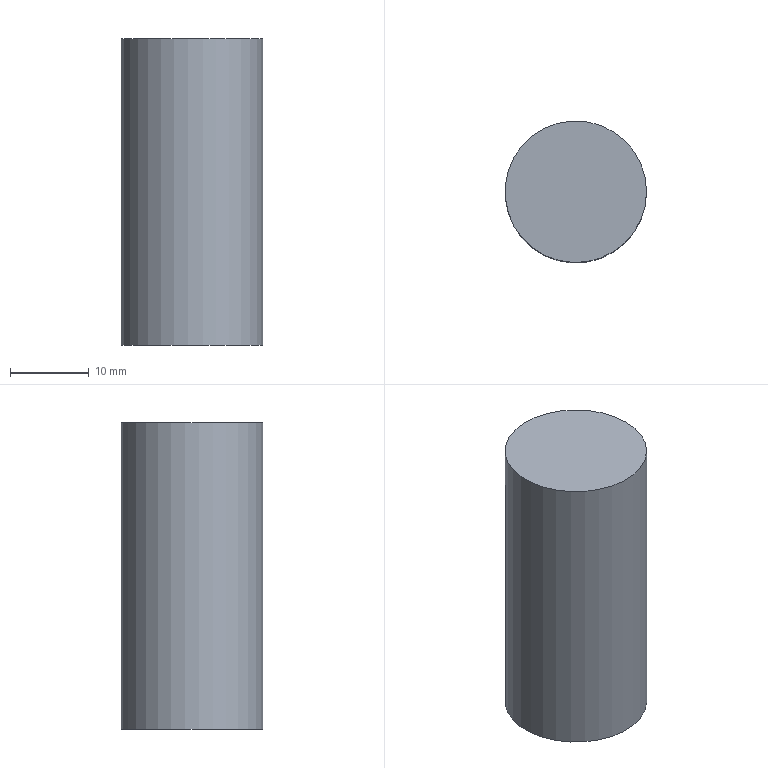Part | STEP file | 1000uf-80V | 1 solid | 3 faces | box 18 x 18 x 39 mm | volume 9924 mm3 | plane 2 | cylinder 1 | commonest cylinder face diameters 18 x1
STEP:
#1=CARTESIAN_POINT('',(0.,0.,0.));
#2=DIRECTION('',(0.,0.,1.));
#3=DIRECTION('',(1.,0.,0.));
#4=AXIS2_PLACEMENT_3D('',#1,#2,#3);
#5=CARTESIAN_POINT('',(9.,0.,39.));
#6=VERTEX_POINT('',#5);
#7=CARTESIAN_POINT('',(0.,0.,39.));
#8=DIRECTION('',(0.,0.,1.));
#9=DIRECTION('',(1.,0.,0.));
#10=AXIS2_PLACEMENT_3D('',#7,#8,#9);
#11=CIRCLE('',#10,9.);
#12=CARTESIAN_POINT('',(0.,0.,39.));
#13=DIRECTION('',(0.,0.,-1.));
#14=DIRECTION('',(-1.,0.,0.));
#15=AXIS2_PLACEMENT_3D('',#12,#13,#14);
#16=CYLINDRICAL_SURFACE('',#15,9.);
#17=CARTESIAN_POINT('',(9.425,0.));
#18=DIRECTION('',(-1.,0.));
#19=VECTOR('',#18,1.);
#20=LINE('',#17,#19);
#21=(GEOMETRIC_REPRESENTATION_CONTEXT(2)PARAMETRIC_REPRESENTATION_CONTEXT()REPRESENTATION_CONTEXT('',''));
#22=DEFINITIONAL_REPRESENTATION('',(#20),#21);
#23=PCURVE('',#16,#22);
#24=CARTESIAN_POINT('',(0.,0.,39.));
#25=DIRECTION('',(0.,0.,1.));
#26=DIRECTION('',(1.,0.,0.));
#27=AXIS2_PLACEMENT_3D('',#24,#25,#26);
#28=PLANE('',#27);
#29=CARTESIAN_POINT('',(0.,0.));
#30=DIRECTION('',(1.,0.));
#31=AXIS2_PLACEMENT_2D('',#29,#30);
#32=CIRCLE('',#31,9.);
#33=(GEOMETRIC_REPRESENTATION_CONTEXT(2)PARAMETRIC_REPRESENTATION_CONTEXT()REPRESENTATION_CONTEXT('',''));
#34=DEFINITIONAL_REPRESENTATION('',(#32),#33);
#35=PCURVE('',#28,#34);
#36=SURFACE_CURVE('',#11,(#23,#35),.PCURVE_S1.);
#37=EDGE_CURVE('',#6,#6,#36,.T.);
#38=ORIENTED_EDGE('',*,*,#37,.F.);
#39=CARTESIAN_POINT('',(9.,0.,0.));
#40=VERTEX_POINT('',#39);
#41=CARTESIAN_POINT('',(9.,0.,39.));
#42=CARTESIAN_POINT('',(9.,0.,0.));
#43=B_SPLINE_CURVE_WITH_KNOTS('',1,(#41,#42),.UNSPECIFIED.,.F.,.F.,(2,2),(0.,39.),.PIECEWISE_BEZIER_KNOTS.);
#44=CARTESIAN_POINT('',(9.425,0.));
#45=DIRECTION('',(0.,1.));
#46=VECTOR('',#45,1.);
#47=LINE('',#44,#46);
#48=(GEOMETRIC_REPRESENTATION_CONTEXT(2)PARAMETRIC_REPRESENTATION_CONTEXT()REPRESENTATION_CONTEXT('',''));
#49=DEFINITIONAL_REPRESENTATION('',(#47),#48);
#50=PCURVE('',#16,#49);
#51=CARTESIAN_POINT('',(3.142,0.));
#52=DIRECTION('',(0.,1.));
#53=VECTOR('',#52,1.);
#54=LINE('',#51,#53);
#55=(GEOMETRIC_REPRESENTATION_CONTEXT(2)PARAMETRIC_REPRESENTATION_CONTEXT()REPRESENTATION_CONTEXT('',''));
#56=DEFINITIONAL_REPRESENTATION('',(#54),#55);
#57=PCURVE('',#16,#56);
#58=SEAM_CURVE('',#43,(#50,#57),.PCURVE_S1.);
#59=EDGE_CURVE('',#6,#40,#58,.T.);
#60=ORIENTED_EDGE('',*,*,#59,.T.);
#61=CARTESIAN_POINT('',(0.,0.,0.));
#62=DIRECTION('',(0.,0.,1.));
#63=DIRECTION('',(1.,0.,0.));
#64=AXIS2_PLACEMENT_3D('',#61,#62,#63);
#65=CIRCLE('',#64,9.);
#66=CARTESIAN_POINT('',(9.425,39.));
#67=DIRECTION('',(-1.,0.));
#68=VECTOR('',#67,1.);
#69=LINE('',#66,#68);
#70=(GEOMETRIC_REPRESENTATION_CONTEXT(2)PARAMETRIC_REPRESENTATION_CONTEXT()REPRESENTATION_CONTEXT('',''));
#71=DEFINITIONAL_REPRESENTATION('',(#69),#70);
#72=PCURVE('',#16,#71);
#73=CARTESIAN_POINT('',(0.,0.,0.));
#74=DIRECTION('',(0.,0.,1.));
#75=DIRECTION('',(1.,0.,0.));
#76=AXIS2_PLACEMENT_3D('',#73,#74,#75);
#77=PLANE('',#76);
#78=CARTESIAN_POINT('',(0.,0.));
#79=DIRECTION('',(1.,0.));
#80=AXIS2_PLACEMENT_2D('',#78,#79);
#81=CIRCLE('',#80,9.);
#82=(GEOMETRIC_REPRESENTATION_CONTEXT(2)PARAMETRIC_REPRESENTATION_CONTEXT()REPRESENTATION_CONTEXT('',''));
#83=DEFINITIONAL_REPRESENTATION('',(#81),#82);
#84=PCURVE('',#77,#83);
#85=SURFACE_CURVE('',#65,(#72,#84),.PCURVE_S1.);
#86=EDGE_CURVE('',#40,#40,#85,.T.);
#87=ORIENTED_EDGE('',*,*,#86,.T.);
#88=ORIENTED_EDGE('',*,*,#59,.F.);
#89=EDGE_LOOP('',(#38,#60,#87,#88));
#90=FACE_BOUND('',#89,.T.);
#91=ADVANCED_FACE('',(#90),#16,.T.);
#92=ORIENTED_EDGE('',*,*,#37,.T.);
#93=EDGE_LOOP('',(#92));
#94=FACE_BOUND('',#93,.T.);
#95=ADVANCED_FACE('',(#94),#28,.T.);
#96=ORIENTED_EDGE('',*,*,#86,.F.);
#97=EDGE_LOOP('',(#96));
#98=FACE_BOUND('',#97,.T.);
#99=ADVANCED_FACE('',(#98),#77,.F.);
#100=CLOSED_SHELL('',(#91,#95,#99));
#101=MANIFOLD_SOLID_BREP('',#100);
#102=(LENGTH_UNIT()NAMED_UNIT(*)SI_UNIT(.MILLI.,.METRE.));
#103=UNCERTAINTY_MEASURE_WITH_UNIT(LENGTH_MEASURE(0.00001),#102,'','');
#104=(NAMED_UNIT(*)PLANE_ANGLE_UNIT()SI_UNIT($,.RADIAN.));
#105=(NAMED_UNIT(*)SI_UNIT($,.STERADIAN.)SOLID_ANGLE_UNIT());
#106=(GEOMETRIC_REPRESENTATION_CONTEXT(3)GLOBAL_UNCERTAINTY_ASSIGNED_CONTEXT((#103))GLOBAL_UNIT_ASSIGNED_CONTEXT((#102,#104,#105))REPRESENTATION_CONTEXT('',''));
#107=ADVANCED_BREP_SHAPE_REPRESENTATION('',(#4,#101),#106);